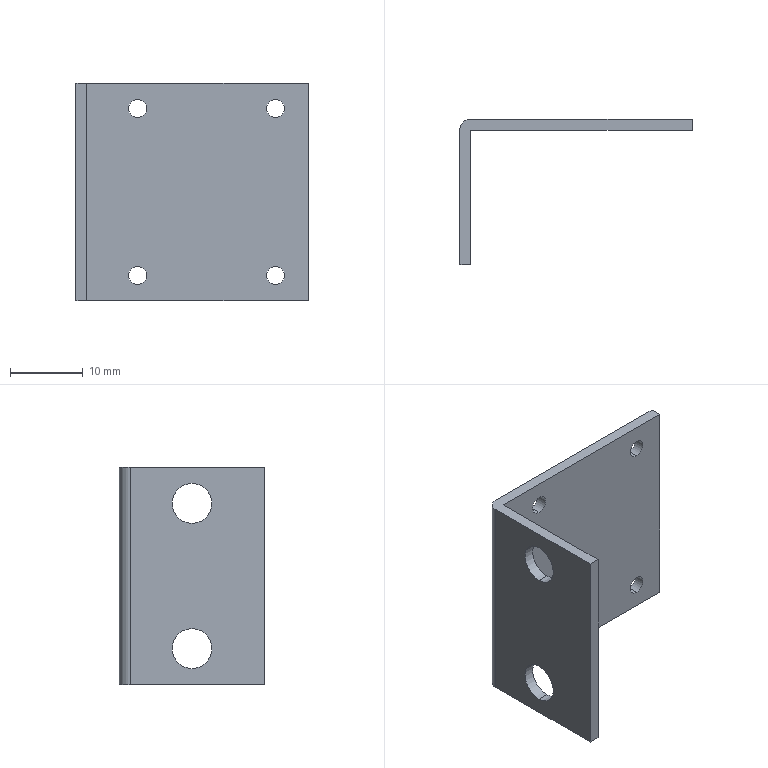Part | STEP file | 0245_203_Blacket | 1 solid | 21 faces | box 32 x 20 x 30 mm | volume 2157 mm3 | cylinder 13 | plane 8 | commonest cylinder face diameters 2.5 x8 5.5 x4 3 x1